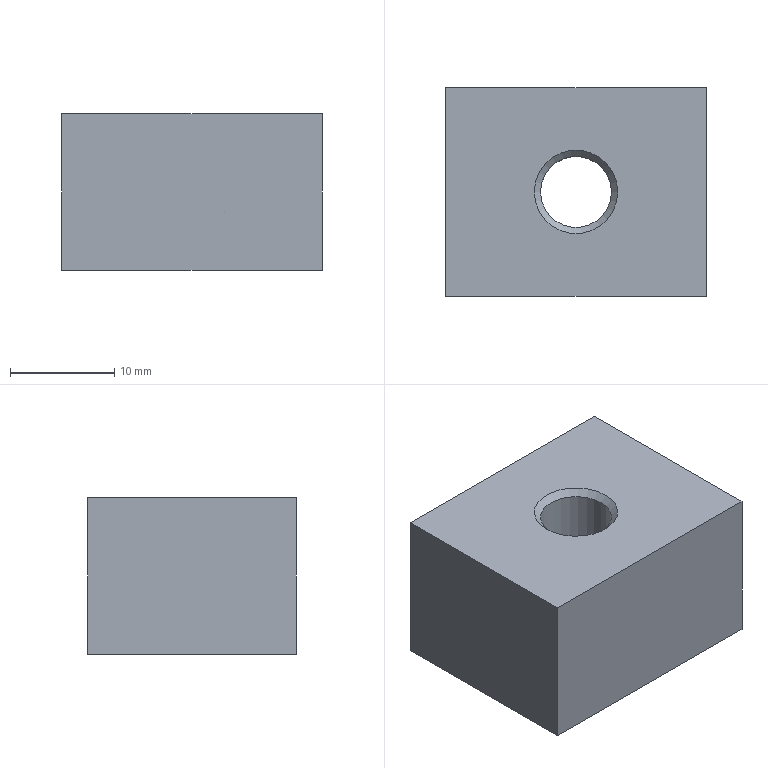Part | NX | features DATUM_CSYS 1, EXTRUDE 1, HOLE PACKAGE 1, SIMPLE HOLE 1, SYMBOLIC_THREAD 1 | 1 solid | 9 faces | box 25 x 20 x 15 mm | volume 6947 mm3 | plane 6 | cone 2 | cylinder 1 | commonest cylinder face diameters 6.8 x1
STEP:
#1=CARTESIAN_POINT('',(-12.5,10.,0.));
#2=VERTEX_POINT('',#1);
#3=CARTESIAN_POINT('',(12.5,10.,0.));
#4=VERTEX_POINT('',#3);
#5=CARTESIAN_POINT('',(-12.5,10.,0.));
#6=DIRECTION('',(1.,0.,0.));
#7=VECTOR('',#6,1000.);
#8=LINE('',#5,#7);
#9=EDGE_CURVE('',#2,#4,#8,.T.);
#10=ORIENTED_EDGE('',*,*,#9,.F.);
#11=CARTESIAN_POINT('',(-12.5,10.,15.));
#12=VERTEX_POINT('',#11);
#13=CARTESIAN_POINT('',(-12.5,10.,15.));
#14=DIRECTION('',(0.,0.,-1.));
#15=VECTOR('',#14,1000.);
#16=LINE('',#13,#15);
#17=EDGE_CURVE('',#12,#2,#16,.T.);
#18=ORIENTED_EDGE('',*,*,#17,.F.);
#19=CARTESIAN_POINT('',(12.5,10.,15.));
#20=VERTEX_POINT('',#19);
#21=CARTESIAN_POINT('',(-12.5,10.,15.));
#22=DIRECTION('',(1.,0.,0.));
#23=VECTOR('',#22,1000.);
#24=LINE('',#21,#23);
#25=EDGE_CURVE('',#12,#20,#24,.T.);
#26=ORIENTED_EDGE('',*,*,#25,.T.);
#27=CARTESIAN_POINT('',(12.5,10.,15.));
#28=DIRECTION('',(0.,0.,-1.));
#29=VECTOR('',#28,1000.);
#30=LINE('',#27,#29);
#31=EDGE_CURVE('',#20,#4,#30,.T.);
#32=ORIENTED_EDGE('',*,*,#31,.T.);
#33=EDGE_LOOP('',(#10,#18,#26,#32));
#34=FACE_BOUND('',#33,.T.);
#35=CARTESIAN_POINT('',(-12.5,10.,15.));
#36=DIRECTION('',(0.,1.,0.));
#37=DIRECTION('',(0.,0.,1.));
#38=AXIS2_PLACEMENT_3D('',#35,#36,#37);
#39=PLANE('',#38);
#40=ADVANCED_FACE('',(#34),#39,.T.);
#41=CARTESIAN_POINT('',(12.5,-10.,0.));
#42=VERTEX_POINT('',#41);
#43=CARTESIAN_POINT('',(12.5,10.,0.));
#44=DIRECTION('',(0.,-1.,0.));
#45=VECTOR('',#44,1000.);
#46=LINE('',#43,#45);
#47=EDGE_CURVE('',#4,#42,#46,.T.);
#48=ORIENTED_EDGE('',*,*,#47,.F.);
#49=ORIENTED_EDGE('',*,*,#31,.F.);
#50=CARTESIAN_POINT('',(12.5,-10.,15.));
#51=VERTEX_POINT('',#50);
#52=CARTESIAN_POINT('',(12.5,10.,15.));
#53=DIRECTION('',(0.,-1.,0.));
#54=VECTOR('',#53,1000.);
#55=LINE('',#52,#54);
#56=EDGE_CURVE('',#20,#51,#55,.T.);
#57=ORIENTED_EDGE('',*,*,#56,.T.);
#58=CARTESIAN_POINT('',(12.5,-10.,15.));
#59=DIRECTION('',(0.,0.,-1.));
#60=VECTOR('',#59,1000.);
#61=LINE('',#58,#60);
#62=EDGE_CURVE('',#51,#42,#61,.T.);
#63=ORIENTED_EDGE('',*,*,#62,.T.);
#64=EDGE_LOOP('',(#48,#49,#57,#63));
#65=FACE_BOUND('',#64,.T.);
#66=CARTESIAN_POINT('',(12.5,10.,15.));
#67=DIRECTION('',(1.,0.,0.));
#68=DIRECTION('',(0.,0.,-1.));
#69=AXIS2_PLACEMENT_3D('',#66,#67,#68);
#70=PLANE('',#69);
#71=ADVANCED_FACE('',(#65),#70,.T.);
#72=CARTESIAN_POINT('',(-12.5,-10.,0.));
#73=VERTEX_POINT('',#72);
#74=CARTESIAN_POINT('',(12.5,-10.,0.));
#75=DIRECTION('',(-1.,0.,0.));
#76=VECTOR('',#75,1000.);
#77=LINE('',#74,#76);
#78=EDGE_CURVE('',#42,#73,#77,.T.);
#79=ORIENTED_EDGE('',*,*,#78,.F.);
#80=ORIENTED_EDGE('',*,*,#62,.F.);
#81=CARTESIAN_POINT('',(-12.5,-10.,15.));
#82=VERTEX_POINT('',#81);
#83=CARTESIAN_POINT('',(12.5,-10.,15.));
#84=DIRECTION('',(-1.,0.,0.));
#85=VECTOR('',#84,1000.);
#86=LINE('',#83,#85);
#87=EDGE_CURVE('',#51,#82,#86,.T.);
#88=ORIENTED_EDGE('',*,*,#87,.T.);
#89=CARTESIAN_POINT('',(-12.5,-10.,15.));
#90=DIRECTION('',(0.,0.,-1.));
#91=VECTOR('',#90,1000.);
#92=LINE('',#89,#91);
#93=EDGE_CURVE('',#82,#73,#92,.T.);
#94=ORIENTED_EDGE('',*,*,#93,.T.);
#95=EDGE_LOOP('',(#79,#80,#88,#94));
#96=FACE_BOUND('',#95,.T.);
#97=CARTESIAN_POINT('',(12.5,-10.,15.));
#98=DIRECTION('',(0.,-1.,0.));
#99=DIRECTION('',(0.,0.,-1.));
#100=AXIS2_PLACEMENT_3D('',#97,#98,#99);
#101=PLANE('',#100);
#102=ADVANCED_FACE('',(#96),#101,.T.);
#103=CARTESIAN_POINT('',(-12.5,-10.,0.));
#104=DIRECTION('',(0.,1.,0.));
#105=VECTOR('',#104,1000.);
#106=LINE('',#103,#105);
#107=EDGE_CURVE('',#73,#2,#106,.T.);
#108=ORIENTED_EDGE('',*,*,#107,.F.);
#109=ORIENTED_EDGE('',*,*,#93,.F.);
#110=CARTESIAN_POINT('',(-12.5,-10.,15.));
#111=DIRECTION('',(0.,1.,0.));
#112=VECTOR('',#111,1000.);
#113=LINE('',#110,#112);
#114=EDGE_CURVE('',#82,#12,#113,.T.);
#115=ORIENTED_EDGE('',*,*,#114,.T.);
#116=ORIENTED_EDGE('',*,*,#17,.T.);
#117=EDGE_LOOP('',(#108,#109,#115,#116));
#118=FACE_BOUND('',#117,.T.);
#119=CARTESIAN_POINT('',(-12.5,-10.,15.));
#120=DIRECTION('',(-1.,0.,0.));
#121=DIRECTION('',(0.,0.,1.));
#122=AXIS2_PLACEMENT_3D('',#119,#120,#121);
#123=PLANE('',#122);
#124=ADVANCED_FACE('',(#118),#123,.T.);
#125=CARTESIAN_POINT('',(-4.,0.,15.));
#126=VERTEX_POINT('',#125);
#127=CARTESIAN_POINT('',(0.,0.,15.));
#128=DIRECTION('',(0.,0.,-1.));
#129=DIRECTION('',(-1.,0.,0.));
#130=AXIS2_PLACEMENT_3D('',#127,#128,#129);
#131=CIRCLE('',#130,4.);
#132=EDGE_CURVE('',#126,#126,#131,.T.);
#133=ORIENTED_EDGE('',*,*,#132,.T.);
#134=EDGE_LOOP('',(#133));
#135=FACE_BOUND('',#134,.T.);
#136=ORIENTED_EDGE('',*,*,#25,.F.);
#137=ORIENTED_EDGE('',*,*,#114,.F.);
#138=ORIENTED_EDGE('',*,*,#87,.F.);
#139=ORIENTED_EDGE('',*,*,#56,.F.);
#140=EDGE_LOOP('',(#136,#137,#138,#139));
#141=FACE_BOUND('',#140,.T.);
#142=CARTESIAN_POINT('',(0.,0.,15.));
#143=DIRECTION('',(0.,0.,-1.));
#144=DIRECTION('',(-1.,0.,0.));
#145=AXIS2_PLACEMENT_3D('',#142,#143,#144);
#146=PLANE('',#145);
#147=ADVANCED_FACE('',(#135,#141),#146,.F.);
#148=CARTESIAN_POINT('',(-4.,0.,0.));
#149=VERTEX_POINT('',#148);
#150=CARTESIAN_POINT('',(0.,0.,0.));
#151=DIRECTION('',(0.,0.,-1.));
#152=DIRECTION('',(-1.,0.,0.));
#153=AXIS2_PLACEMENT_3D('',#150,#151,#152);
#154=CIRCLE('',#153,4.);
#155=EDGE_CURVE('',#149,#149,#154,.F.);
#156=ORIENTED_EDGE('',*,*,#155,.T.);
#157=EDGE_LOOP('',(#156));
#158=FACE_BOUND('',#157,.T.);
#159=ORIENTED_EDGE('',*,*,#9,.T.);
#160=ORIENTED_EDGE('',*,*,#47,.T.);
#161=ORIENTED_EDGE('',*,*,#78,.T.);
#162=ORIENTED_EDGE('',*,*,#107,.T.);
#163=EDGE_LOOP('',(#159,#160,#161,#162));
#164=FACE_BOUND('',#163,.T.);
#165=CARTESIAN_POINT('',(0.,0.,0.));
#166=DIRECTION('',(0.,0.,-1.));
#167=DIRECTION('',(-1.,0.,0.));
#168=AXIS2_PLACEMENT_3D('',#165,#166,#167);
#169=PLANE('',#168);
#170=ADVANCED_FACE('',(#158,#164),#169,.T.);
#171=CARTESIAN_POINT('',(-3.4,0.,14.4));
#172=VERTEX_POINT('',#171);
#173=CARTESIAN_POINT('',(0.,0.,14.4));
#174=DIRECTION('',(0.,0.,-1.));
#175=DIRECTION('',(-1.,0.,0.));
#176=AXIS2_PLACEMENT_3D('',#173,#174,#175);
#177=CIRCLE('',#176,3.4);
#178=EDGE_CURVE('',#172,#172,#177,.F.);
#179=ORIENTED_EDGE('',*,*,#178,.T.);
#180=EDGE_LOOP('',(#179));
#181=FACE_BOUND('',#180,.T.);
#182=CARTESIAN_POINT('',(-3.4,0.,0.6));
#183=VERTEX_POINT('',#182);
#184=CARTESIAN_POINT('',(0.,0.,0.6));
#185=DIRECTION('',(0.,0.,-1.));
#186=DIRECTION('',(-1.,0.,0.));
#187=AXIS2_PLACEMENT_3D('',#184,#185,#186);
#188=CIRCLE('',#187,3.4);
#189=EDGE_CURVE('',#183,#183,#188,.T.);
#190=ORIENTED_EDGE('',*,*,#189,.T.);
#191=EDGE_LOOP('',(#190));
#192=FACE_BOUND('',#191,.T.);
#193=CARTESIAN_POINT('',(0.,0.,0.));
#194=DIRECTION('',(0.,0.,1.));
#195=DIRECTION('',(1.,0.,0.));
#196=AXIS2_PLACEMENT_3D('',#193,#194,#195);
#197=CYLINDRICAL_SURFACE('',#196,3.4);
#198=ADVANCED_FACE('',(#181,#192),#197,.F.);
#199=ORIENTED_EDGE('',*,*,#189,.F.);
#200=EDGE_LOOP('',(#199));
#201=FACE_BOUND('',#200,.T.);
#202=ORIENTED_EDGE('',*,*,#155,.F.);
#203=EDGE_LOOP('',(#202));
#204=FACE_BOUND('',#203,.T.);
#205=CARTESIAN_POINT('',(0.,0.,0.));
#206=DIRECTION('',(0.,0.,-1.));
#207=DIRECTION('',(-1.,0.,0.));
#208=AXIS2_PLACEMENT_3D('',#205,#206,#207);
#209=CONICAL_SURFACE('',#208,4.,0.7854);
#210=ADVANCED_FACE('',(#201,#204),#209,.F.);
#211=ORIENTED_EDGE('',*,*,#178,.F.);
#212=EDGE_LOOP('',(#211));
#213=FACE_BOUND('',#212,.T.);
#214=ORIENTED_EDGE('',*,*,#132,.F.);
#215=EDGE_LOOP('',(#214));
#216=FACE_BOUND('',#215,.T.);
#217=CARTESIAN_POINT('',(0.,0.,15.));
#218=DIRECTION('',(0.,0.,1.));
#219=DIRECTION('',(1.,0.,0.));
#220=AXIS2_PLACEMENT_3D('',#217,#218,#219);
#221=CONICAL_SURFACE('',#220,4.,0.7854);
#222=ADVANCED_FACE('',(#213,#216),#221,.F.);
#223=CLOSED_SHELL('',(#40,#71,#102,#124,#147,#170,#198,#210,#222));
#224=MANIFOLD_SOLID_BREP('',#223);
#225=(LENGTH_UNIT()NAMED_UNIT(*)SI_UNIT(.MILLI.,.METRE.));
#226=UNCERTAINTY_MEASURE_WITH_UNIT(LENGTH_MEASURE(0.00001),#225,'','');
#227=(NAMED_UNIT(*)PLANE_ANGLE_UNIT()SI_UNIT($,.RADIAN.));
#228=(NAMED_UNIT(*)SI_UNIT($,.STERADIAN.)SOLID_ANGLE_UNIT());
#229=(GEOMETRIC_REPRESENTATION_CONTEXT(3)GLOBAL_UNCERTAINTY_ASSIGNED_CONTEXT((#226))GLOBAL_UNIT_ASSIGNED_CONTEXT((#225,#227,#228))REPRESENTATION_CONTEXT('',''));
#230=ADVANCED_BREP_SHAPE_REPRESENTATION('',(#224),#229);